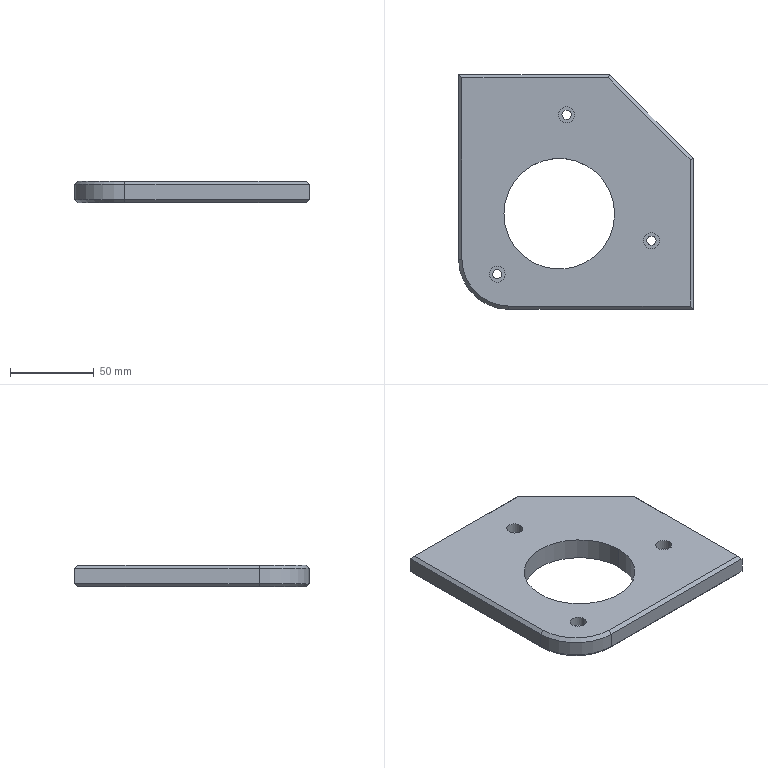Part | Creo | 1 solid | 37 faces | box 140 x 140 x 13 mm | volume 187737 mm3 | plane 20 | cylinder 15 | cone 2 | commonest cylinder face diameters 5.5 x6 9.5 x6 66 x2 60 x1
STEP:
#1=CARTESIAN_POINT('',(284.172,372.995,-24.));
#2=VERTEX_POINT('',#1);
#3=CARTESIAN_POINT('',(197.,372.995,-24.));
#4=VERTEX_POINT('',#3);
#5=CARTESIAN_POINT('',(284.172,372.995,-24.));
#6=DIRECTION('',(-1.,0.,0.));
#7=VECTOR('',#6,87.172);
#8=LINE('',#5,#7);
#9=EDGE_CURVE('',#2,#4,#8,.T.);
#10=ORIENTED_EDGE('',*,*,#9,.T.);
#11=CARTESIAN_POINT('',(197.,264.995,-24.));
#12=VERTEX_POINT('',#11);
#13=CARTESIAN_POINT('',(197.,372.995,-24.));
#14=DIRECTION('',(0.,-1.,0.));
#15=VECTOR('',#14,108.);
#16=LINE('',#13,#15);
#17=EDGE_CURVE('',#4,#12,#16,.T.);
#18=ORIENTED_EDGE('',*,*,#17,.T.);
#19=CARTESIAN_POINT('',(225.,236.995,-24.));
#20=VERTEX_POINT('',#19);
#21=CARTESIAN_POINT('',(225.,264.995,-24.));
#22=DIRECTION('',(0.,0.,-1.));
#23=DIRECTION('',(0.,-1.,0.));
#24=AXIS2_PLACEMENT_3D('',#21,#22,#23);
#25=CIRCLE('',#24,28.);
#26=EDGE_CURVE('',#20,#12,#25,.T.);
#27=ORIENTED_EDGE('',*,*,#26,.F.);
#28=CARTESIAN_POINT('',(333.,236.995,-24.));
#29=VERTEX_POINT('',#28);
#30=CARTESIAN_POINT('',(225.,236.995,-24.));
#31=DIRECTION('',(1.,0.,0.));
#32=VECTOR('',#31,108.);
#33=LINE('',#30,#32);
#34=EDGE_CURVE('',#20,#29,#33,.T.);
#35=ORIENTED_EDGE('',*,*,#34,.T.);
#36=CARTESIAN_POINT('',(333.,324.167,-24.));
#37=VERTEX_POINT('',#36);
#38=CARTESIAN_POINT('',(333.,236.995,-24.));
#39=DIRECTION('',(0.,1.,0.));
#40=VECTOR('',#39,87.172);
#41=LINE('',#38,#40);
#42=EDGE_CURVE('',#29,#37,#41,.T.);
#43=ORIENTED_EDGE('',*,*,#42,.T.);
#44=CARTESIAN_POINT('',(284.172,372.995,-24.));
#45=DIRECTION('',(0.7071,-0.7071,0.));
#46=VECTOR('',#45,69.054);
#47=LINE('',#44,#46);
#48=EDGE_CURVE('',#2,#37,#47,.T.);
#49=ORIENTED_EDGE('',*,*,#48,.F.);
#50=EDGE_LOOP('',(#10,#18,#27,#35,#43,#49));
#51=FACE_OUTER_BOUND('',#50,.F.);
#52=CARTESIAN_POINT('',(307.25,276.,-24.));
#53=VERTEX_POINT('',#52);
#54=CARTESIAN_POINT('',(312.75,276.,-24.));
#55=VERTEX_POINT('',#54);
#56=CARTESIAN_POINT('',(310.,276.,-24.));
#57=DIRECTION('',(0.,0.,1.));
#58=DIRECTION('',(-1.,0.,0.));
#59=AXIS2_PLACEMENT_3D('',#56,#57,#58);
#60=CIRCLE('',#59,2.75);
#61=EDGE_CURVE('',#53,#55,#60,.T.);
#62=ORIENTED_EDGE('',*,*,#61,.F.);
#63=CARTESIAN_POINT('',(310.,276.,-24.));
#64=DIRECTION('',(0.,0.,1.));
#65=DIRECTION('',(1.,0.,0.));
#66=AXIS2_PLACEMENT_3D('',#63,#64,#65);
#67=CIRCLE('',#66,2.75);
#68=EDGE_CURVE('',#55,#53,#67,.T.);
#69=ORIENTED_EDGE('',*,*,#68,.F.);
#70=EDGE_LOOP('',(#62,#69));
#71=FACE_BOUND('',#70,.F.);
#72=CARTESIAN_POINT('',(256.618,351.,-24.));
#73=VERTEX_POINT('',#72);
#74=CARTESIAN_POINT('',(262.118,351.,-24.));
#75=VERTEX_POINT('',#74);
#76=CARTESIAN_POINT('',(259.368,351.,-24.));
#77=DIRECTION('',(0.,0.,1.));
#78=DIRECTION('',(-1.,0.,0.));
#79=AXIS2_PLACEMENT_3D('',#76,#77,#78);
#80=CIRCLE('',#79,2.75);
#81=EDGE_CURVE('',#73,#75,#80,.T.);
#82=ORIENTED_EDGE('',*,*,#81,.F.);
#83=CARTESIAN_POINT('',(259.368,351.,-24.));
#84=DIRECTION('',(0.,0.,1.));
#85=DIRECTION('',(1.,0.,0.));
#86=AXIS2_PLACEMENT_3D('',#83,#84,#85);
#87=CIRCLE('',#86,2.75);
#88=EDGE_CURVE('',#75,#73,#87,.T.);
#89=ORIENTED_EDGE('',*,*,#88,.F.);
#90=EDGE_LOOP('',(#82,#89));
#91=FACE_BOUND('',#90,.F.);
#92=CARTESIAN_POINT('',(215.25,256.,-24.));
#93=VERTEX_POINT('',#92);
#94=CARTESIAN_POINT('',(220.75,256.,-24.));
#95=VERTEX_POINT('',#94);
#96=CARTESIAN_POINT('',(218.,256.,-24.));
#97=DIRECTION('',(0.,0.,1.));
#98=DIRECTION('',(-1.,0.,0.));
#99=AXIS2_PLACEMENT_3D('',#96,#97,#98);
#100=CIRCLE('',#99,2.75);
#101=EDGE_CURVE('',#93,#95,#100,.T.);
#102=ORIENTED_EDGE('',*,*,#101,.F.);
#103=CARTESIAN_POINT('',(218.,256.,-24.));
#104=DIRECTION('',(0.,0.,1.));
#105=DIRECTION('',(1.,0.,0.));
#106=AXIS2_PLACEMENT_3D('',#103,#104,#105);
#107=CIRCLE('',#106,2.75);
#108=EDGE_CURVE('',#95,#93,#107,.T.);
#109=ORIENTED_EDGE('',*,*,#108,.F.);
#110=EDGE_LOOP('',(#102,#109));
#111=FACE_BOUND('',#110,.F.);
#112=CARTESIAN_POINT('',(222.,291.995,-24.));
#113=VERTEX_POINT('',#112);
#114=CARTESIAN_POINT('',(288.,291.995,-24.));
#115=VERTEX_POINT('',#114);
#116=CARTESIAN_POINT('',(255.,291.995,-24.));
#117=DIRECTION('',(0.,0.,1.));
#118=DIRECTION('',(-1.,0.,0.));
#119=AXIS2_PLACEMENT_3D('',#116,#117,#118);
#120=CIRCLE('',#119,33.);
#121=EDGE_CURVE('',#113,#115,#120,.T.);
#122=ORIENTED_EDGE('',*,*,#121,.F.);
#123=CARTESIAN_POINT('',(255.,291.995,-24.));
#124=DIRECTION('',(0.,0.,1.));
#125=DIRECTION('',(1.,0.,0.));
#126=AXIS2_PLACEMENT_3D('',#123,#124,#125);
#127=CIRCLE('',#126,33.);
#128=EDGE_CURVE('',#115,#113,#127,.T.);
#129=ORIENTED_EDGE('',*,*,#128,.F.);
#130=EDGE_LOOP('',(#122,#129));
#131=FACE_BOUND('',#130,.F.);
#132=CARTESIAN_POINT('',(265.,302.495,-24.));
#133=DIRECTION('',(0.,0.,-1.));
#134=DIRECTION('',(-1.,0.,0.));
#135=AXIS2_PLACEMENT_3D('',#132,#133,#134);
#136=PLANE('',#135);
#137=ADVANCED_FACE('',(#51,#71,#91,#111,#131),#136,.T.);
#138=CARTESIAN_POINT('',(195.,374.995,-22.));
#139=VERTEX_POINT('',#138);
#140=CARTESIAN_POINT('',(195.,374.995,-22.));
#141=DIRECTION('',(0.5774,-0.5774,-0.5774));
#142=VECTOR('',#141,3.464);
#143=LINE('',#140,#142);
#144=EDGE_CURVE('',#139,#4,#143,.T.);
#145=ORIENTED_EDGE('',*,*,#144,.T.);
#146=ORIENTED_EDGE('',*,*,#9,.F.);
#147=CARTESIAN_POINT('',(285.,374.995,-22.));
#148=VERTEX_POINT('',#147);
#149=CARTESIAN_POINT('',(285.,374.995,-22.));
#150=DIRECTION('',(-0.2811,-0.6786,-0.6786));
#151=VECTOR('',#150,2.947);
#152=LINE('',#149,#151);
#153=EDGE_CURVE('',#148,#2,#152,.T.);
#154=ORIENTED_EDGE('',*,*,#153,.F.);
#155=CARTESIAN_POINT('',(195.,374.995,-22.));
#156=DIRECTION('',(1.,0.,0.));
#157=VECTOR('',#156,90.);
#158=LINE('',#155,#157);
#159=EDGE_CURVE('',#139,#148,#158,.T.);
#160=ORIENTED_EDGE('',*,*,#159,.F.);
#161=EDGE_LOOP('',(#145,#146,#154,#160));
#162=FACE_OUTER_BOUND('',#161,.F.);
#163=CARTESIAN_POINT('',(265.,372.995,-24.));
#164=DIRECTION('',(0.,-0.7071,0.7071));
#165=DIRECTION('',(1.,0.,0.));
#166=AXIS2_PLACEMENT_3D('',#163,#164,#165);
#167=PLANE('',#166);
#168=ADVANCED_FACE('',(#162),#167,.F.);
#169=CARTESIAN_POINT('',(195.,264.995,-22.));
#170=VERTEX_POINT('',#169);
#171=CARTESIAN_POINT('',(195.,264.995,-22.));
#172=DIRECTION('',(0.7071,0.,-0.7071));
#173=VECTOR('',#172,2.828);
#174=LINE('',#171,#173);
#175=EDGE_CURVE('',#170,#12,#174,.T.);
#176=ORIENTED_EDGE('',*,*,#175,.T.);
#177=ORIENTED_EDGE('',*,*,#17,.F.);
#178=ORIENTED_EDGE('',*,*,#144,.F.);
#179=CARTESIAN_POINT('',(195.,264.995,-22.));
#180=DIRECTION('',(0.,1.,0.));
#181=VECTOR('',#180,110.);
#182=LINE('',#179,#181);
#183=EDGE_CURVE('',#170,#139,#182,.T.);
#184=ORIENTED_EDGE('',*,*,#183,.F.);
#185=EDGE_LOOP('',(#176,#177,#178,#184));
#186=FACE_OUTER_BOUND('',#185,.F.);
#187=CARTESIAN_POINT('',(197.,302.495,-24.));
#188=DIRECTION('',(0.7071,0.,0.7071));
#189=DIRECTION('',(0.,1.,0.));
#190=AXIS2_PLACEMENT_3D('',#187,#188,#189);
#191=PLANE('',#190);
#192=ADVANCED_FACE('',(#186),#191,.F.);
#193=ORIENTED_EDGE('',*,*,#175,.F.);
#194=CARTESIAN_POINT('',(225.,234.995,-22.));
#195=VERTEX_POINT('',#194);
#196=CARTESIAN_POINT('',(225.,264.995,-22.));
#197=DIRECTION('',(0.,0.,-1.));
#198=DIRECTION('',(0.,-1.,0.));
#199=AXIS2_PLACEMENT_3D('',#196,#197,#198);
#200=CIRCLE('',#199,30.);
#201=EDGE_CURVE('',#195,#170,#200,.T.);
#202=ORIENTED_EDGE('',*,*,#201,.F.);
#203=CARTESIAN_POINT('',(225.,236.995,-24.));
#204=DIRECTION('',(0.,-0.7071,0.7071));
#205=VECTOR('',#204,2.828);
#206=LINE('',#203,#205);
#207=EDGE_CURVE('',#20,#195,#206,.T.);
#208=ORIENTED_EDGE('',*,*,#207,.F.);
#209=ORIENTED_EDGE('',*,*,#26,.T.);
#210=EDGE_LOOP('',(#193,#202,#208,#209));
#211=FACE_OUTER_BOUND('',#210,.F.);
#212=CARTESIAN_POINT('',(225.,264.995,-23.));
#213=DIRECTION('',(0.,0.,1.));
#214=DIRECTION('',(1.,0.,0.));
#215=AXIS2_PLACEMENT_3D('',#212,#213,#214);
#216=CONICAL_SURFACE('',#215,29.,45.);
#217=ADVANCED_FACE('',(#211),#216,.T.);
#218=CARTESIAN_POINT('',(225.,234.995,-13.));
#219=VERTEX_POINT('',#218);
#220=CARTESIAN_POINT('',(225.,234.995,-22.));
#221=DIRECTION('',(0.,0.,1.));
#222=VECTOR('',#221,9.);
#223=LINE('',#220,#222);
#224=EDGE_CURVE('',#195,#219,#223,.T.);
#225=ORIENTED_EDGE('',*,*,#224,.F.);
#226=ORIENTED_EDGE('',*,*,#201,.T.);
#227=CARTESIAN_POINT('',(195.,264.995,-13.));
#228=VERTEX_POINT('',#227);
#229=CARTESIAN_POINT('',(195.,264.995,-13.));
#230=DIRECTION('',(0.,0.,-1.));
#231=VECTOR('',#230,9.);
#232=LINE('',#229,#231);
#233=EDGE_CURVE('',#228,#170,#232,.T.);
#234=ORIENTED_EDGE('',*,*,#233,.F.);
#235=CARTESIAN_POINT('',(225.,264.995,-13.));
#236=DIRECTION('',(0.,0.,1.));
#237=DIRECTION('',(-1.,0.,0.));
#238=AXIS2_PLACEMENT_3D('',#235,#236,#237);
#239=CIRCLE('',#238,30.);
#240=EDGE_CURVE('',#228,#219,#239,.T.);
#241=ORIENTED_EDGE('',*,*,#240,.T.);
#242=EDGE_LOOP('',(#225,#226,#234,#241));
#243=FACE_OUTER_BOUND('',#242,.F.);
#244=CARTESIAN_POINT('',(225.,264.995,-11.));
#245=DIRECTION('',(0.,0.,-1.));
#246=DIRECTION('',(-1.,0.,0.));
#247=AXIS2_PLACEMENT_3D('',#244,#245,#246);
#248=CYLINDRICAL_SURFACE('',#247,30.);
#249=ADVANCED_FACE('',(#243),#248,.T.);
#250=CARTESIAN_POINT('',(335.,234.995,-22.));
#251=VERTEX_POINT('',#250);
#252=CARTESIAN_POINT('',(335.,234.995,-13.));
#253=VERTEX_POINT('',#252);
#254=CARTESIAN_POINT('',(335.,234.995,-22.));
#255=DIRECTION('',(0.,0.,1.));
#256=VECTOR('',#255,9.);
#257=LINE('',#254,#256);
#258=EDGE_CURVE('',#251,#253,#257,.T.);
#259=ORIENTED_EDGE('',*,*,#258,.F.);
#260=CARTESIAN_POINT('',(335.,234.995,-22.));
#261=DIRECTION('',(-1.,0.,0.));
#262=VECTOR('',#261,110.);
#263=LINE('',#260,#262);
#264=EDGE_CURVE('',#251,#195,#263,.T.);
#265=ORIENTED_EDGE('',*,*,#264,.T.);
#266=ORIENTED_EDGE('',*,*,#224,.T.);
#267=CARTESIAN_POINT('',(225.,234.995,-13.));
#268=DIRECTION('',(1.,0.,0.));
#269=VECTOR('',#268,110.);
#270=LINE('',#267,#269);
#271=EDGE_CURVE('',#219,#253,#270,.T.);
#272=ORIENTED_EDGE('',*,*,#271,.T.);
#273=EDGE_LOOP('',(#259,#265,#266,#272));
#274=FACE_OUTER_BOUND('',#273,.F.);
#275=CARTESIAN_POINT('',(265.,234.995,-11.));
#276=DIRECTION('',(0.,-1.,0.));
#277=DIRECTION('',(0.,0.,-1.));
#278=AXIS2_PLACEMENT_3D('',#275,#276,#277);
#279=PLANE('',#278);
#280=ADVANCED_FACE('',(#274),#279,.T.);
#281=CARTESIAN_POINT('',(335.,324.995,-13.));
#282=VERTEX_POINT('',#281);
#283=CARTESIAN_POINT('',(335.,324.995,-22.));
#284=VERTEX_POINT('',#283);
#285=CARTESIAN_POINT('',(335.,324.995,-13.));
#286=DIRECTION('',(0.,0.,-1.));
#287=VECTOR('',#286,9.);
#288=LINE('',#285,#287);
#289=EDGE_CURVE('',#282,#284,#288,.T.);
#290=ORIENTED_EDGE('',*,*,#289,.T.);
#291=CARTESIAN_POINT('',(335.,324.995,-22.));
#292=DIRECTION('',(0.,-1.,0.));
#293=VECTOR('',#292,90.);
#294=LINE('',#291,#293);
#295=EDGE_CURVE('',#284,#251,#294,.T.);
#296=ORIENTED_EDGE('',*,*,#295,.T.);
#297=ORIENTED_EDGE('',*,*,#258,.T.);
#298=CARTESIAN_POINT('',(335.,234.995,-13.));
#299=DIRECTION('',(0.,1.,0.));
#300=VECTOR('',#299,90.);
#301=LINE('',#298,#300);
#302=EDGE_CURVE('',#253,#282,#301,.T.);
#303=ORIENTED_EDGE('',*,*,#302,.T.);
#304=EDGE_LOOP('',(#290,#296,#297,#303));
#305=FACE_OUTER_BOUND('',#304,.F.);
#306=CARTESIAN_POINT('',(335.,-0.004699,-22.));
#307=DIRECTION('',(-1.,0.,0.));
#308=DIRECTION('',(0.,1.,0.));
#309=AXIS2_PLACEMENT_3D('',#306,#307,#308);
#310=PLANE('',#309);
#311=ADVANCED_FACE('',(#305),#310,.F.);
#312=CARTESIAN_POINT('',(285.,374.995,-13.));
#313=VERTEX_POINT('',#312);
#314=CARTESIAN_POINT('',(285.,374.995,-22.));
#315=DIRECTION('',(0.,0.,1.));
#316=VECTOR('',#315,9.);
#317=LINE('',#314,#316);
#318=EDGE_CURVE('',#148,#313,#317,.T.);
#319=ORIENTED_EDGE('',*,*,#318,.F.);
#320=CARTESIAN_POINT('',(285.,374.995,-22.));
#321=DIRECTION('',(0.7071,-0.7071,0.));
#322=VECTOR('',#321,70.711);
#323=LINE('',#320,#322);
#324=EDGE_CURVE('',#148,#284,#323,.T.);
#325=ORIENTED_EDGE('',*,*,#324,.T.);
#326=ORIENTED_EDGE('',*,*,#289,.F.);
#327=CARTESIAN_POINT('',(335.,324.995,-13.));
#328=DIRECTION('',(-0.7071,0.7071,0.));
#329=VECTOR('',#328,70.711);
#330=LINE('',#327,#329);
#331=EDGE_CURVE('',#282,#313,#330,.T.);
#332=ORIENTED_EDGE('',*,*,#331,.T.);
#333=EDGE_LOOP('',(#319,#325,#326,#332));
#334=FACE_OUTER_BOUND('',#333,.F.);
#335=CARTESIAN_POINT('',(285.,374.995,-187.));
#336=DIRECTION('',(0.7071,0.7071,0.));
#337=DIRECTION('',(0.,0.,1.));
#338=AXIS2_PLACEMENT_3D('',#335,#336,#337);
#339=PLANE('',#338);
#340=ADVANCED_FACE('',(#334),#339,.T.);
#341=CARTESIAN_POINT('',(195.,374.995,-13.));
#342=VERTEX_POINT('',#341);
#343=CARTESIAN_POINT('',(195.,374.995,-22.));
#344=DIRECTION('',(0.,0.,1.));
#345=VECTOR('',#344,9.);
#346=LINE('',#343,#345);
#347=EDGE_CURVE('',#139,#342,#346,.T.);
#348=ORIENTED_EDGE('',*,*,#347,.F.);
#349=ORIENTED_EDGE('',*,*,#159,.T.);
#350=ORIENTED_EDGE('',*,*,#318,.T.);
#351=CARTESIAN_POINT('',(285.,374.995,-13.));
#352=DIRECTION('',(-1.,0.,0.));
#353=VECTOR('',#352,90.);
#354=LINE('',#351,#353);
#355=EDGE_CURVE('',#313,#342,#354,.T.);
#356=ORIENTED_EDGE('',*,*,#355,.T.);
#357=EDGE_LOOP('',(#348,#349,#350,#356));
#358=FACE_OUTER_BOUND('',#357,.F.);
#359=CARTESIAN_POINT('',(285.,374.995,-187.));
#360=DIRECTION('',(0.,1.,0.));
#361=DIRECTION('',(0.,0.,1.));
#362=AXIS2_PLACEMENT_3D('',#359,#360,#361);
#363=PLANE('',#362);
#364=ADVANCED_FACE('',(#358),#363,.T.);
#365=ORIENTED_EDGE('',*,*,#233,.T.);
#366=ORIENTED_EDGE('',*,*,#183,.T.);
#367=ORIENTED_EDGE('',*,*,#347,.T.);
#368=CARTESIAN_POINT('',(195.,374.995,-13.));
#369=DIRECTION('',(0.,-1.,0.));
#370=VECTOR('',#369,110.);
#371=LINE('',#368,#370);
#372=EDGE_CURVE('',#342,#228,#371,.T.);
#373=ORIENTED_EDGE('',*,*,#372,.T.);
#374=EDGE_LOOP('',(#365,#366,#367,#373));
#375=FACE_OUTER_BOUND('',#374,.F.);
#376=CARTESIAN_POINT('',(195.,302.495,-11.));
#377=DIRECTION('',(-1.,0.,0.));
#378=DIRECTION('',(0.,0.,1.));
#379=AXIS2_PLACEMENT_3D('',#376,#377,#378);
#380=PLANE('',#379);
#381=ADVANCED_FACE('',(#375),#380,.T.);
#382=CARTESIAN_POINT('',(197.,264.995,-11.));
#383=VERTEX_POINT('',#382);
#384=CARTESIAN_POINT('',(197.,264.995,-11.));
#385=DIRECTION('',(-0.7071,0.,-0.7071));
#386=VECTOR('',#385,2.828);
#387=LINE('',#384,#386);
#388=EDGE_CURVE('',#383,#228,#387,.T.);
#389=ORIENTED_EDGE('',*,*,#388,.T.);
#390=ORIENTED_EDGE('',*,*,#372,.F.);
#391=CARTESIAN_POINT('',(197.,372.995,-11.));
#392=VERTEX_POINT('',#391);
#393=CARTESIAN_POINT('',(197.,372.995,-11.));
#394=DIRECTION('',(-0.5774,0.5774,-0.5774));
#395=VECTOR('',#394,3.464);
#396=LINE('',#393,#395);
#397=EDGE_CURVE('',#392,#342,#396,.T.);
#398=ORIENTED_EDGE('',*,*,#397,.F.);
#399=CARTESIAN_POINT('',(197.,264.995,-11.));
#400=DIRECTION('',(0.,1.,0.));
#401=VECTOR('',#400,108.);
#402=LINE('',#399,#401);
#403=EDGE_CURVE('',#383,#392,#402,.T.);
#404=ORIENTED_EDGE('',*,*,#403,.F.);
#405=EDGE_LOOP('',(#389,#390,#398,#404));
#406=FACE_OUTER_BOUND('',#405,.F.);
#407=CARTESIAN_POINT('',(197.,302.495,-11.));
#408=DIRECTION('',(0.7071,0.,-0.7071));
#409=DIRECTION('',(0.,-1.,0.));
#410=AXIS2_PLACEMENT_3D('',#407,#408,#409);
#411=PLANE('',#410);
#412=ADVANCED_FACE('',(#406),#411,.F.);
#413=ORIENTED_EDGE('',*,*,#388,.F.);
#414=CARTESIAN_POINT('',(225.,236.995,-11.));
#415=VERTEX_POINT('',#414);
#416=CARTESIAN_POINT('',(225.,264.995,-11.));
#417=DIRECTION('',(0.,0.,1.));
#418=DIRECTION('',(-1.,0.,0.));
#419=AXIS2_PLACEMENT_3D('',#416,#417,#418);
#420=CIRCLE('',#419,28.);
#421=EDGE_CURVE('',#383,#415,#420,.T.);
#422=ORIENTED_EDGE('',*,*,#421,.T.);
#423=CARTESIAN_POINT('',(225.,234.995,-13.));
#424=DIRECTION('',(0.,0.7071,0.7071));
#425=VECTOR('',#424,2.828);
#426=LINE('',#423,#425);
#427=EDGE_CURVE('',#219,#415,#426,.T.);
#428=ORIENTED_EDGE('',*,*,#427,.F.);
#429=ORIENTED_EDGE('',*,*,#240,.F.);
#430=EDGE_LOOP('',(#413,#422,#428,#429));
#431=FACE_OUTER_BOUND('',#430,.F.);
#432=CARTESIAN_POINT('',(225.,264.995,-12.));
#433=DIRECTION('',(0.,0.,-1.));
#434=DIRECTION('',(-1.,0.,0.));
#435=AXIS2_PLACEMENT_3D('',#432,#433,#434);
#436=CONICAL_SURFACE('',#435,29.,45.);
#437=ADVANCED_FACE('',(#431),#436,.T.);
#438=CARTESIAN_POINT('',(333.,324.167,-11.));
#439=VERTEX_POINT('',#438);
#440=CARTESIAN_POINT('',(333.,236.995,-11.));
#441=VERTEX_POINT('',#440);
#442=CARTESIAN_POINT('',(333.,324.167,-11.));
#443=DIRECTION('',(0.,-1.,0.));
#444=VECTOR('',#443,87.172);
#445=LINE('',#442,#444);
#446=EDGE_CURVE('',#439,#441,#445,.T.);
#447=ORIENTED_EDGE('',*,*,#446,.T.);
#448=CARTESIAN_POINT('',(333.,236.995,-11.));
#449=DIRECTION('',(-1.,0.,0.));
#450=VECTOR('',#449,108.);
#451=LINE('',#448,#450);
#452=EDGE_CURVE('',#441,#415,#451,.T.);
#453=ORIENTED_EDGE('',*,*,#452,.T.);
#454=ORIENTED_EDGE('',*,*,#421,.F.);
#455=ORIENTED_EDGE('',*,*,#403,.T.);
#456=CARTESIAN_POINT('',(284.172,372.995,-11.));
#457=VERTEX_POINT('',#456);
#458=CARTESIAN_POINT('',(197.,372.995,-11.));
#459=DIRECTION('',(1.,0.,0.));
#460=VECTOR('',#459,87.172);
#461=LINE('',#458,#460);
#462=EDGE_CURVE('',#392,#457,#461,.T.);
#463=ORIENTED_EDGE('',*,*,#462,.T.);
#464=CARTESIAN_POINT('',(333.,324.167,-11.));
#465=DIRECTION('',(-0.7071,0.7071,0.));
#466=VECTOR('',#465,69.054);
#467=LINE('',#464,#466);
#468=EDGE_CURVE('',#439,#457,#467,.T.);
#469=ORIENTED_EDGE('',*,*,#468,.F.);
#470=EDGE_LOOP('',(#447,#453,#454,#455,#463,#469));
#471=FACE_OUTER_BOUND('',#470,.F.);
#472=CARTESIAN_POINT('',(314.75,276.,-11.));
#473=VERTEX_POINT('',#472);
#474=CARTESIAN_POINT('',(305.25,276.,-11.));
#475=VERTEX_POINT('',#474);
#476=CARTESIAN_POINT('',(310.,276.,-11.));
#477=DIRECTION('',(0.,0.,-1.));
#478=DIRECTION('',(1.,0.,0.));
#479=AXIS2_PLACEMENT_3D('',#476,#477,#478);
#480=CIRCLE('',#479,4.75);
#481=EDGE_CURVE('',#473,#475,#480,.T.);
#482=ORIENTED_EDGE('',*,*,#481,.F.);
#483=CARTESIAN_POINT('',(310.,276.,-11.));
#484=DIRECTION('',(0.,0.,-1.));
#485=DIRECTION('',(-1.,0.,0.));
#486=AXIS2_PLACEMENT_3D('',#483,#484,#485);
#487=CIRCLE('',#486,4.75);
#488=EDGE_CURVE('',#475,#473,#487,.T.);
#489=ORIENTED_EDGE('',*,*,#488,.F.);
#490=EDGE_LOOP('',(#482,#489));
#491=FACE_BOUND('',#490,.F.);
#492=CARTESIAN_POINT('',(264.118,351.,-11.));
#493=VERTEX_POINT('',#492);
#494=CARTESIAN_POINT('',(254.618,351.,-11.));
#495=VERTEX_POINT('',#494);
#496=CARTESIAN_POINT('',(259.368,351.,-11.));
#497=DIRECTION('',(0.,0.,-1.));
#498=DIRECTION('',(1.,0.,0.));
#499=AXIS2_PLACEMENT_3D('',#496,#497,#498);
#500=CIRCLE('',#499,4.75);
#501=EDGE_CURVE('',#493,#495,#500,.T.);
#502=ORIENTED_EDGE('',*,*,#501,.F.);
#503=CARTESIAN_POINT('',(259.368,351.,-11.));
#504=DIRECTION('',(0.,0.,-1.));
#505=DIRECTION('',(-1.,0.,0.));
#506=AXIS2_PLACEMENT_3D('',#503,#504,#505);
#507=CIRCLE('',#506,4.75);
#508=EDGE_CURVE('',#495,#493,#507,.T.);
#509=ORIENTED_EDGE('',*,*,#508,.F.);
#510=EDGE_LOOP('',(#502,#509));
#511=FACE_BOUND('',#510,.F.);
#512=CARTESIAN_POINT('',(222.75,256.,-11.));
#513=VERTEX_POINT('',#512);
#514=CARTESIAN_POINT('',(213.25,256.,-11.));
#515=VERTEX_POINT('',#514);
#516=CARTESIAN_POINT('',(218.,256.,-11.));
#517=DIRECTION('',(0.,0.,-1.));
#518=DIRECTION('',(1.,0.,0.));
#519=AXIS2_PLACEMENT_3D('',#516,#517,#518);
#520=CIRCLE('',#519,4.75);
#521=EDGE_CURVE('',#513,#515,#520,.T.);
#522=ORIENTED_EDGE('',*,*,#521,.F.);
#523=CARTESIAN_POINT('',(218.,256.,-11.));
#524=DIRECTION('',(0.,0.,-1.));
#525=DIRECTION('',(-1.,0.,0.));
#526=AXIS2_PLACEMENT_3D('',#523,#524,#525);
#527=CIRCLE('',#526,4.75);
#528=EDGE_CURVE('',#515,#513,#527,.T.);
#529=ORIENTED_EDGE('',*,*,#528,.F.);
#530=EDGE_LOOP('',(#522,#529));
#531=FACE_BOUND('',#530,.F.);
#532=CARTESIAN_POINT('',(288.,291.995,-11.));
#533=VERTEX_POINT('',#532);
#534=CARTESIAN_POINT('',(222.,291.995,-11.));
#535=VERTEX_POINT('',#534);
#536=CARTESIAN_POINT('',(255.,291.995,-11.));
#537=DIRECTION('',(0.,0.,-1.));
#538=DIRECTION('',(1.,0.,0.));
#539=AXIS2_PLACEMENT_3D('',#536,#537,#538);
#540=CIRCLE('',#539,33.);
#541=EDGE_CURVE('',#533,#535,#540,.T.);
#542=ORIENTED_EDGE('',*,*,#541,.F.);
#543=CARTESIAN_POINT('',(255.,291.995,-11.));
#544=DIRECTION('',(0.,0.,-1.));
#545=DIRECTION('',(-1.,0.,0.));
#546=AXIS2_PLACEMENT_3D('',#543,#544,#545);
#547=CIRCLE('',#546,33.);
#548=EDGE_CURVE('',#535,#533,#547,.T.);
#549=ORIENTED_EDGE('',*,*,#548,.F.);
#550=EDGE_LOOP('',(#542,#549));
#551=FACE_BOUND('',#550,.F.);
#552=CARTESIAN_POINT('',(265.,302.495,-11.));
#553=DIRECTION('',(0.,0.,1.));
#554=DIRECTION('',(1.,0.,0.));
#555=AXIS2_PLACEMENT_3D('',#552,#553,#554);
#556=PLANE('',#555);
#557=ADVANCED_FACE('',(#471,#491,#511,#531,#551),#556,.T.);
#558=CARTESIAN_POINT('',(335.,234.995,-13.));
#559=DIRECTION('',(-0.5774,0.5774,0.5774));
#560=VECTOR('',#559,3.464);
#561=LINE('',#558,#560);
#562=EDGE_CURVE('',#253,#441,#561,.T.);
#563=ORIENTED_EDGE('',*,*,#562,.T.);
#564=ORIENTED_EDGE('',*,*,#446,.F.);
#565=CARTESIAN_POINT('',(335.,324.995,-13.));
#566=DIRECTION('',(-0.6786,-0.2811,0.6786));
#567=VECTOR('',#566,2.947);
#568=LINE('',#565,#567);
#569=EDGE_CURVE('',#282,#439,#568,.T.);
#570=ORIENTED_EDGE('',*,*,#569,.F.);
#571=ORIENTED_EDGE('',*,*,#302,.F.);
#572=EDGE_LOOP('',(#563,#564,#570,#571));
#573=FACE_OUTER_BOUND('',#572,.F.);
#574=CARTESIAN_POINT('',(333.,302.495,-11.));
#575=DIRECTION('',(0.7071,0.,0.7071));
#576=DIRECTION('',(0.,-1.,0.));
#577=AXIS2_PLACEMENT_3D('',#574,#575,#576);
#578=PLANE('',#577);
#579=ADVANCED_FACE('',(#573),#578,.T.);
#580=ORIENTED_EDGE('',*,*,#427,.T.);
#581=ORIENTED_EDGE('',*,*,#452,.F.);
#582=ORIENTED_EDGE('',*,*,#562,.F.);
#583=ORIENTED_EDGE('',*,*,#271,.F.);
#584=EDGE_LOOP('',(#580,#581,#582,#583));
#585=FACE_OUTER_BOUND('',#584,.F.);
#586=CARTESIAN_POINT('',(265.,236.995,-11.));
#587=DIRECTION('',(0.,0.7071,-0.7071));
#588=DIRECTION('',(1.,0.,0.));
#589=AXIS2_PLACEMENT_3D('',#586,#587,#588);
#590=PLANE('',#589);
#591=ADVANCED_FACE('',(#585),#590,.F.);
#592=ORIENTED_EDGE('',*,*,#569,.T.);
#593=ORIENTED_EDGE('',*,*,#468,.T.);
#594=CARTESIAN_POINT('',(284.172,372.995,-11.));
#595=DIRECTION('',(0.2811,0.6786,-0.6786));
#596=VECTOR('',#595,2.947);
#597=LINE('',#594,#596);
#598=EDGE_CURVE('',#457,#313,#597,.T.);
#599=ORIENTED_EDGE('',*,*,#598,.T.);
#600=ORIENTED_EDGE('',*,*,#331,.F.);
#601=EDGE_LOOP('',(#592,#593,#599,#600));
#602=FACE_OUTER_BOUND('',#601,.F.);
#603=CARTESIAN_POINT('',(309.836,347.331,-11.));
#604=DIRECTION('',(-0.5,-0.5,-0.7071));
#605=DIRECTION('',(-0.7071,0.7071,0.));
#606=AXIS2_PLACEMENT_3D('',#603,#604,#605);
#607=PLANE('',#606);
#608=ADVANCED_FACE('',(#602),#607,.F.);
#609=ORIENTED_EDGE('',*,*,#397,.T.);
#610=ORIENTED_EDGE('',*,*,#355,.F.);
#611=ORIENTED_EDGE('',*,*,#598,.F.);
#612=ORIENTED_EDGE('',*,*,#462,.F.);
#613=EDGE_LOOP('',(#609,#610,#611,#612));
#614=FACE_OUTER_BOUND('',#613,.F.);
#615=CARTESIAN_POINT('',(265.,372.995,-11.));
#616=DIRECTION('',(0.,-0.7071,-0.7071));
#617=DIRECTION('',(-1.,0.,0.));
#618=AXIS2_PLACEMENT_3D('',#615,#616,#617);
#619=PLANE('',#618);
#620=ADVANCED_FACE('',(#614),#619,.F.);
#621=CARTESIAN_POINT('',(305.25,276.,-17.));
#622=VERTEX_POINT('',#621);
#623=CARTESIAN_POINT('',(314.75,276.,-17.));
#624=VERTEX_POINT('',#623);
#625=CARTESIAN_POINT('',(310.,276.,-17.));
#626=DIRECTION('',(0.,0.,1.));
#627=DIRECTION('',(-1.,0.,0.));
#628=AXIS2_PLACEMENT_3D('',#625,#626,#627);
#629=CIRCLE('',#628,4.75);
#630=EDGE_CURVE('',#622,#624,#629,.T.);
#631=ORIENTED_EDGE('',*,*,#630,.T.);
#632=CARTESIAN_POINT('',(314.75,276.,-17.));
#633=DIRECTION('',(0.,0.,1.));
#634=VECTOR('',#633,6.);
#635=LINE('',#632,#634);
#636=EDGE_CURVE('',#624,#473,#635,.T.);
#637=ORIENTED_EDGE('',*,*,#636,.T.);
#638=ORIENTED_EDGE('',*,*,#481,.T.);
#639=CARTESIAN_POINT('',(305.25,276.,-17.));
#640=DIRECTION('',(0.,0.,1.));
#641=VECTOR('',#640,6.);
#642=LINE('',#639,#641);
#643=EDGE_CURVE('',#622,#475,#642,.T.);
#644=ORIENTED_EDGE('',*,*,#643,.F.);
#645=EDGE_LOOP('',(#631,#637,#638,#644));
#646=FACE_OUTER_BOUND('',#645,.F.);
#647=CARTESIAN_POINT('',(310.,276.,-11.));
#648=DIRECTION('',(0.,0.,1.));
#649=DIRECTION('',(1.,0.,0.));
#650=AXIS2_PLACEMENT_3D('',#647,#648,#649);
#651=CYLINDRICAL_SURFACE('',#650,4.75);
#652=ADVANCED_FACE('',(#646),#651,.F.);
#653=CARTESIAN_POINT('',(310.,276.,-17.));
#654=DIRECTION('',(0.,0.,1.));
#655=DIRECTION('',(1.,0.,0.));
#656=AXIS2_PLACEMENT_3D('',#653,#654,#655);
#657=CIRCLE('',#656,4.75);
#658=EDGE_CURVE('',#624,#622,#657,.T.);
#659=ORIENTED_EDGE('',*,*,#658,.F.);
#660=ORIENTED_EDGE('',*,*,#630,.F.);
#661=EDGE_LOOP('',(#659,#660));
#662=FACE_OUTER_BOUND('',#661,.F.);
#663=CARTESIAN_POINT('',(312.75,276.,-17.));
#664=VERTEX_POINT('',#663);
#665=CARTESIAN_POINT('',(307.25,276.,-17.));
#666=VERTEX_POINT('',#665);
#667=CARTESIAN_POINT('',(310.,276.,-17.));
#668=DIRECTION('',(0.,0.,-1.));
#669=DIRECTION('',(1.,0.,0.));
#670=AXIS2_PLACEMENT_3D('',#667,#668,#669);
#671=CIRCLE('',#670,2.75);
#672=EDGE_CURVE('',#664,#666,#671,.T.);
#673=ORIENTED_EDGE('',*,*,#672,.F.);
#674=CARTESIAN_POINT('',(310.,276.,-17.));
#675=DIRECTION('',(0.,0.,-1.));
#676=DIRECTION('',(-1.,0.,0.));
#677=AXIS2_PLACEMENT_3D('',#674,#675,#676);
#678=CIRCLE('',#677,2.75);
#679=EDGE_CURVE('',#666,#664,#678,.T.);
#680=ORIENTED_EDGE('',*,*,#679,.F.);
#681=EDGE_LOOP('',(#673,#680));
#682=FACE_BOUND('',#681,.F.);
#683=CARTESIAN_POINT('',(310.,280.75,-17.));
#684=DIRECTION('',(0.,0.,-1.));
#685=DIRECTION('',(-1.,0.,0.));
#686=AXIS2_PLACEMENT_3D('',#683,#684,#685);
#687=PLANE('',#686);
#688=ADVANCED_FACE('',(#662,#682),#687,.F.);
#689=ORIENTED_EDGE('',*,*,#61,.T.);
#690=CARTESIAN_POINT('',(312.75,276.,-24.));
#691=DIRECTION('',(0.,0.,1.));
#692=VECTOR('',#691,7.);
#693=LINE('',#690,#692);
#694=EDGE_CURVE('',#55,#664,#693,.T.);
#695=ORIENTED_EDGE('',*,*,#694,.T.);
#696=ORIENTED_EDGE('',*,*,#672,.T.);
#697=CARTESIAN_POINT('',(307.25,276.,-24.));
#698=DIRECTION('',(0.,0.,1.));
#699=VECTOR('',#698,7.);
#700=LINE('',#697,#699);
#701=EDGE_CURVE('',#53,#666,#700,.T.);
#702=ORIENTED_EDGE('',*,*,#701,.F.);
#703=EDGE_LOOP('',(#689,#695,#696,#702));
#704=FACE_OUTER_BOUND('',#703,.F.);
#705=CARTESIAN_POINT('',(310.,276.,-11.));
#706=DIRECTION('',(0.,0.,1.));
#707=DIRECTION('',(1.,0.,0.));
#708=AXIS2_PLACEMENT_3D('',#705,#706,#707);
#709=CYLINDRICAL_SURFACE('',#708,2.75);
#710=ADVANCED_FACE('',(#704),#709,.F.);
#711=ORIENTED_EDGE('',*,*,#68,.T.);
#712=ORIENTED_EDGE('',*,*,#701,.T.);
#713=ORIENTED_EDGE('',*,*,#679,.T.);
#714=ORIENTED_EDGE('',*,*,#694,.F.);
#715=EDGE_LOOP('',(#711,#712,#713,#714));
#716=FACE_OUTER_BOUND('',#715,.F.);
#717=CARTESIAN_POINT('',(310.,276.,-11.));
#718=DIRECTION('',(0.,0.,1.));
#719=DIRECTION('',(1.,0.,0.));
#720=AXIS2_PLACEMENT_3D('',#717,#718,#719);
#721=CYLINDRICAL_SURFACE('',#720,2.75);
#722=ADVANCED_FACE('',(#716),#721,.F.);
#723=ORIENTED_EDGE('',*,*,#658,.T.);
#724=ORIENTED_EDGE('',*,*,#643,.T.);
#725=ORIENTED_EDGE('',*,*,#488,.T.);
#726=ORIENTED_EDGE('',*,*,#636,.F.);
#727=EDGE_LOOP('',(#723,#724,#725,#726));
#728=FACE_OUTER_BOUND('',#727,.F.);
#729=CARTESIAN_POINT('',(310.,276.,-11.));
#730=DIRECTION('',(0.,0.,1.));
#731=DIRECTION('',(1.,0.,0.));
#732=AXIS2_PLACEMENT_3D('',#729,#730,#731);
#733=CYLINDRICAL_SURFACE('',#732,4.75);
#734=ADVANCED_FACE('',(#728),#733,.F.);
#735=CARTESIAN_POINT('',(254.618,351.,-17.));
#736=VERTEX_POINT('',#735);
#737=CARTESIAN_POINT('',(264.118,351.,-17.));
#738=VERTEX_POINT('',#737);
#739=CARTESIAN_POINT('',(259.368,351.,-17.));
#740=DIRECTION('',(0.,0.,1.));
#741=DIRECTION('',(-1.,0.,0.));
#742=AXIS2_PLACEMENT_3D('',#739,#740,#741);
#743=CIRCLE('',#742,4.75);
#744=EDGE_CURVE('',#736,#738,#743,.T.);
#745=ORIENTED_EDGE('',*,*,#744,.T.);
#746=CARTESIAN_POINT('',(264.118,351.,-17.));
#747=DIRECTION('',(0.,0.,1.));
#748=VECTOR('',#747,6.);
#749=LINE('',#746,#748);
#750=EDGE_CURVE('',#738,#493,#749,.T.);
#751=ORIENTED_EDGE('',*,*,#750,.T.);
#752=ORIENTED_EDGE('',*,*,#501,.T.);
#753=CARTESIAN_POINT('',(254.618,351.,-17.));
#754=DIRECTION('',(0.,0.,1.));
#755=VECTOR('',#754,6.);
#756=LINE('',#753,#755);
#757=EDGE_CURVE('',#736,#495,#756,.T.);
#758=ORIENTED_EDGE('',*,*,#757,.F.);
#759=EDGE_LOOP('',(#745,#751,#752,#758));
#760=FACE_OUTER_BOUND('',#759,.F.);
#761=CARTESIAN_POINT('',(259.368,351.,-11.));
#762=DIRECTION('',(0.,0.,1.));
#763=DIRECTION('',(1.,0.,0.));
#764=AXIS2_PLACEMENT_3D('',#761,#762,#763);
#765=CYLINDRICAL_SURFACE('',#764,4.75);
#766=ADVANCED_FACE('',(#760),#765,.F.);
#767=CARTESIAN_POINT('',(259.368,351.,-17.));
#768=DIRECTION('',(0.,0.,1.));
#769=DIRECTION('',(1.,0.,0.));
#770=AXIS2_PLACEMENT_3D('',#767,#768,#769);
#771=CIRCLE('',#770,4.75);
#772=EDGE_CURVE('',#738,#736,#771,.T.);
#773=ORIENTED_EDGE('',*,*,#772,.F.);
#774=ORIENTED_EDGE('',*,*,#744,.F.);
#775=EDGE_LOOP('',(#773,#774));
#776=FACE_OUTER_BOUND('',#775,.F.);
#777=CARTESIAN_POINT('',(262.118,351.,-17.));
#778=VERTEX_POINT('',#777);
#779=CARTESIAN_POINT('',(256.618,351.,-17.));
#780=VERTEX_POINT('',#779);
#781=CARTESIAN_POINT('',(259.368,351.,-17.));
#782=DIRECTION('',(0.,0.,-1.));
#783=DIRECTION('',(1.,0.,0.));
#784=AXIS2_PLACEMENT_3D('',#781,#782,#783);
#785=CIRCLE('',#784,2.75);
#786=EDGE_CURVE('',#778,#780,#785,.T.);
#787=ORIENTED_EDGE('',*,*,#786,.F.);
#788=CARTESIAN_POINT('',(259.368,351.,-17.));
#789=DIRECTION('',(0.,0.,-1.));
#790=DIRECTION('',(-1.,0.,0.));
#791=AXIS2_PLACEMENT_3D('',#788,#789,#790);
#792=CIRCLE('',#791,2.75);
#793=EDGE_CURVE('',#780,#778,#792,.T.);
#794=ORIENTED_EDGE('',*,*,#793,.F.);
#795=EDGE_LOOP('',(#787,#794));
#796=FACE_BOUND('',#795,.F.);
#797=CARTESIAN_POINT('',(259.368,355.75,-17.));
#798=DIRECTION('',(0.,0.,-1.));
#799=DIRECTION('',(-1.,0.,0.));
#800=AXIS2_PLACEMENT_3D('',#797,#798,#799);
#801=PLANE('',#800);
#802=ADVANCED_FACE('',(#776,#796),#801,.F.);
#803=ORIENTED_EDGE('',*,*,#81,.T.);
#804=CARTESIAN_POINT('',(262.118,351.,-24.));
#805=DIRECTION('',(0.,0.,1.));
#806=VECTOR('',#805,7.);
#807=LINE('',#804,#806);
#808=EDGE_CURVE('',#75,#778,#807,.T.);
#809=ORIENTED_EDGE('',*,*,#808,.T.);
#810=ORIENTED_EDGE('',*,*,#786,.T.);
#811=CARTESIAN_POINT('',(256.618,351.,-24.));
#812=DIRECTION('',(0.,0.,1.));
#813=VECTOR('',#812,7.);
#814=LINE('',#811,#813);
#815=EDGE_CURVE('',#73,#780,#814,.T.);
#816=ORIENTED_EDGE('',*,*,#815,.F.);
#817=EDGE_LOOP('',(#803,#809,#810,#816));
#818=FACE_OUTER_BOUND('',#817,.F.);
#819=CARTESIAN_POINT('',(259.368,351.,-11.));
#820=DIRECTION('',(0.,0.,1.));
#821=DIRECTION('',(1.,0.,0.));
#822=AXIS2_PLACEMENT_3D('',#819,#820,#821);
#823=CYLINDRICAL_SURFACE('',#822,2.75);
#824=ADVANCED_FACE('',(#818),#823,.F.);
#825=ORIENTED_EDGE('',*,*,#88,.T.);
#826=ORIENTED_EDGE('',*,*,#815,.T.);
#827=ORIENTED_EDGE('',*,*,#793,.T.);
#828=ORIENTED_EDGE('',*,*,#808,.F.);
#829=EDGE_LOOP('',(#825,#826,#827,#828));
#830=FACE_OUTER_BOUND('',#829,.F.);
#831=CARTESIAN_POINT('',(259.368,351.,-11.));
#832=DIRECTION('',(0.,0.,1.));
#833=DIRECTION('',(1.,0.,0.));
#834=AXIS2_PLACEMENT_3D('',#831,#832,#833);
#835=CYLINDRICAL_SURFACE('',#834,2.75);
#836=ADVANCED_FACE('',(#830),#835,.F.);
#837=ORIENTED_EDGE('',*,*,#772,.T.);
#838=ORIENTED_EDGE('',*,*,#757,.T.);
#839=ORIENTED_EDGE('',*,*,#508,.T.);
#840=ORIENTED_EDGE('',*,*,#750,.F.);
#841=EDGE_LOOP('',(#837,#838,#839,#840));
#842=FACE_OUTER_BOUND('',#841,.F.);
#843=CARTESIAN_POINT('',(259.368,351.,-11.));
#844=DIRECTION('',(0.,0.,1.));
#845=DIRECTION('',(1.,0.,0.));
#846=AXIS2_PLACEMENT_3D('',#843,#844,#845);
#847=CYLINDRICAL_SURFACE('',#846,4.75);
#848=ADVANCED_FACE('',(#842),#847,.F.);
#849=CARTESIAN_POINT('',(213.25,256.,-17.));
#850=VERTEX_POINT('',#849);
#851=CARTESIAN_POINT('',(222.75,256.,-17.));
#852=VERTEX_POINT('',#851);
#853=CARTESIAN_POINT('',(218.,256.,-17.));
#854=DIRECTION('',(0.,0.,1.));
#855=DIRECTION('',(-1.,0.,0.));
#856=AXIS2_PLACEMENT_3D('',#853,#854,#855);
#857=CIRCLE('',#856,4.75);
#858=EDGE_CURVE('',#850,#852,#857,.T.);
#859=ORIENTED_EDGE('',*,*,#858,.T.);
#860=CARTESIAN_POINT('',(222.75,256.,-17.));
#861=DIRECTION('',(0.,0.,1.));
#862=VECTOR('',#861,6.);
#863=LINE('',#860,#862);
#864=EDGE_CURVE('',#852,#513,#863,.T.);
#865=ORIENTED_EDGE('',*,*,#864,.T.);
#866=ORIENTED_EDGE('',*,*,#521,.T.);
#867=CARTESIAN_POINT('',(213.25,256.,-17.));
#868=DIRECTION('',(0.,0.,1.));
#869=VECTOR('',#868,6.);
#870=LINE('',#867,#869);
#871=EDGE_CURVE('',#850,#515,#870,.T.);
#872=ORIENTED_EDGE('',*,*,#871,.F.);
#873=EDGE_LOOP('',(#859,#865,#866,#872));
#874=FACE_OUTER_BOUND('',#873,.F.);
#875=CARTESIAN_POINT('',(218.,256.,-11.));
#876=DIRECTION('',(0.,0.,1.));
#877=DIRECTION('',(1.,0.,0.));
#878=AXIS2_PLACEMENT_3D('',#875,#876,#877);
#879=CYLINDRICAL_SURFACE('',#878,4.75);
#880=ADVANCED_FACE('',(#874),#879,.F.);
#881=CARTESIAN_POINT('',(218.,256.,-17.));
#882=DIRECTION('',(0.,0.,1.));
#883=DIRECTION('',(1.,0.,0.));
#884=AXIS2_PLACEMENT_3D('',#881,#882,#883);
#885=CIRCLE('',#884,4.75);
#886=EDGE_CURVE('',#852,#850,#885,.T.);
#887=ORIENTED_EDGE('',*,*,#886,.F.);
#888=ORIENTED_EDGE('',*,*,#858,.F.);
#889=EDGE_LOOP('',(#887,#888));
#890=FACE_OUTER_BOUND('',#889,.F.);
#891=CARTESIAN_POINT('',(220.75,256.,-17.));
#892=VERTEX_POINT('',#891);
#893=CARTESIAN_POINT('',(215.25,256.,-17.));
#894=VERTEX_POINT('',#893);
#895=CARTESIAN_POINT('',(218.,256.,-17.));
#896=DIRECTION('',(0.,0.,-1.));
#897=DIRECTION('',(1.,0.,0.));
#898=AXIS2_PLACEMENT_3D('',#895,#896,#897);
#899=CIRCLE('',#898,2.75);
#900=EDGE_CURVE('',#892,#894,#899,.T.);
#901=ORIENTED_EDGE('',*,*,#900,.F.);
#902=CARTESIAN_POINT('',(218.,256.,-17.));
#903=DIRECTION('',(0.,0.,-1.));
#904=DIRECTION('',(-1.,0.,0.));
#905=AXIS2_PLACEMENT_3D('',#902,#903,#904);
#906=CIRCLE('',#905,2.75);
#907=EDGE_CURVE('',#894,#892,#906,.T.);
#908=ORIENTED_EDGE('',*,*,#907,.F.);
#909=EDGE_LOOP('',(#901,#908));
#910=FACE_BOUND('',#909,.F.);
#911=CARTESIAN_POINT('',(218.,260.75,-17.));
#912=DIRECTION('',(0.,0.,-1.));
#913=DIRECTION('',(-1.,0.,0.));
#914=AXIS2_PLACEMENT_3D('',#911,#912,#913);
#915=PLANE('',#914);
#916=ADVANCED_FACE('',(#890,#910),#915,.F.);
#917=ORIENTED_EDGE('',*,*,#101,.T.);
#918=CARTESIAN_POINT('',(220.75,256.,-24.));
#919=DIRECTION('',(0.,0.,1.));
#920=VECTOR('',#919,7.);
#921=LINE('',#918,#920);
#922=EDGE_CURVE('',#95,#892,#921,.T.);
#923=ORIENTED_EDGE('',*,*,#922,.T.);
#924=ORIENTED_EDGE('',*,*,#900,.T.);
#925=CARTESIAN_POINT('',(215.25,256.,-24.));
#926=DIRECTION('',(0.,0.,1.));
#927=VECTOR('',#926,7.);
#928=LINE('',#925,#927);
#929=EDGE_CURVE('',#93,#894,#928,.T.);
#930=ORIENTED_EDGE('',*,*,#929,.F.);
#931=EDGE_LOOP('',(#917,#923,#924,#930));
#932=FACE_OUTER_BOUND('',#931,.F.);
#933=CARTESIAN_POINT('',(218.,256.,-11.));
#934=DIRECTION('',(0.,0.,1.));
#935=DIRECTION('',(1.,0.,0.));
#936=AXIS2_PLACEMENT_3D('',#933,#934,#935);
#937=CYLINDRICAL_SURFACE('',#936,2.75);
#938=ADVANCED_FACE('',(#932),#937,.F.);
#939=ORIENTED_EDGE('',*,*,#108,.T.);
#940=ORIENTED_EDGE('',*,*,#929,.T.);
#941=ORIENTED_EDGE('',*,*,#907,.T.);
#942=ORIENTED_EDGE('',*,*,#922,.F.);
#943=EDGE_LOOP('',(#939,#940,#941,#942));
#944=FACE_OUTER_BOUND('',#943,.F.);
#945=CARTESIAN_POINT('',(218.,256.,-11.));
#946=DIRECTION('',(0.,0.,1.));
#947=DIRECTION('',(1.,0.,0.));
#948=AXIS2_PLACEMENT_3D('',#945,#946,#947);
#949=CYLINDRICAL_SURFACE('',#948,2.75);
#950=ADVANCED_FACE('',(#944),#949,.F.);
#951=ORIENTED_EDGE('',*,*,#886,.T.);
#952=ORIENTED_EDGE('',*,*,#871,.T.);
#953=ORIENTED_EDGE('',*,*,#528,.T.);
#954=ORIENTED_EDGE('',*,*,#864,.F.);
#955=EDGE_LOOP('',(#951,#952,#953,#954));
#956=FACE_OUTER_BOUND('',#955,.F.);
#957=CARTESIAN_POINT('',(218.,256.,-11.));
#958=DIRECTION('',(0.,0.,1.));
#959=DIRECTION('',(1.,0.,0.));
#960=AXIS2_PLACEMENT_3D('',#957,#958,#959);
#961=CYLINDRICAL_SURFACE('',#960,4.75);
#962=ADVANCED_FACE('',(#956),#961,.F.);
#963=ORIENTED_EDGE('',*,*,#541,.T.);
#964=CARTESIAN_POINT('',(222.,291.995,-11.));
#965=DIRECTION('',(0.,0.,-1.));
#966=VECTOR('',#965,13.);
#967=LINE('',#964,#966);
#968=EDGE_CURVE('',#535,#113,#967,.T.);
#969=ORIENTED_EDGE('',*,*,#968,.T.);
#970=ORIENTED_EDGE('',*,*,#121,.T.);
#971=CARTESIAN_POINT('',(288.,291.995,-11.));
#972=DIRECTION('',(0.,0.,-1.));
#973=VECTOR('',#972,13.);
#974=LINE('',#971,#973);
#975=EDGE_CURVE('',#533,#115,#974,.T.);
#976=ORIENTED_EDGE('',*,*,#975,.F.);
#977=EDGE_LOOP('',(#963,#969,#970,#976));
#978=FACE_OUTER_BOUND('',#977,.F.);
#979=CARTESIAN_POINT('',(255.,291.995,-201.));
#980=DIRECTION('',(0.,0.,-1.));
#981=DIRECTION('',(1.,0.,0.));
#982=AXIS2_PLACEMENT_3D('',#979,#980,#981);
#983=CYLINDRICAL_SURFACE('',#982,33.);
#984=ADVANCED_FACE('',(#978),#983,.F.);
#985=ORIENTED_EDGE('',*,*,#548,.T.);
#986=ORIENTED_EDGE('',*,*,#975,.T.);
#987=ORIENTED_EDGE('',*,*,#128,.T.);
#988=ORIENTED_EDGE('',*,*,#968,.F.);
#989=EDGE_LOOP('',(#985,#986,#987,#988));
#990=FACE_OUTER_BOUND('',#989,.F.);
#991=CARTESIAN_POINT('',(255.,291.995,-201.));
#992=DIRECTION('',(0.,0.,-1.));
#993=DIRECTION('',(1.,0.,0.));
#994=AXIS2_PLACEMENT_3D('',#991,#992,#993);
#995=CYLINDRICAL_SURFACE('',#994,33.);
#996=ADVANCED_FACE('',(#990),#995,.F.);
#997=ORIENTED_EDGE('',*,*,#153,.T.);
#998=ORIENTED_EDGE('',*,*,#48,.T.);
#999=CARTESIAN_POINT('',(335.,324.995,-22.));
#1000=DIRECTION('',(-0.6786,-0.2811,-0.6786));
#1001=VECTOR('',#1000,2.947);
#1002=LINE('',#999,#1001);
#1003=EDGE_CURVE('',#284,#37,#1002,.T.);
#1004=ORIENTED_EDGE('',*,*,#1003,.F.);
#1005=ORIENTED_EDGE('',*,*,#324,.F.);
#1006=EDGE_LOOP('',(#997,#998,#1004,#1005));
#1007=FACE_OUTER_BOUND('',#1006,.F.);
#1008=CARTESIAN_POINT('',(309.836,347.331,-24.));
#1009=DIRECTION('',(-0.5,-0.5,0.7071));
#1010=DIRECTION('',(0.7071,-0.7071,0.));
#1011=AXIS2_PLACEMENT_3D('',#1008,#1009,#1010);
#1012=PLANE('',#1011);
#1013=ADVANCED_FACE('',(#1007),#1012,.F.);
#1014=ORIENTED_EDGE('',*,*,#1003,.T.);
#1015=ORIENTED_EDGE('',*,*,#42,.F.);
#1016=CARTESIAN_POINT('',(333.,236.995,-24.));
#1017=DIRECTION('',(0.5774,-0.5774,0.5774));
#1018=VECTOR('',#1017,3.464);
#1019=LINE('',#1016,#1018);
#1020=EDGE_CURVE('',#29,#251,#1019,.T.);
#1021=ORIENTED_EDGE('',*,*,#1020,.T.);
#1022=ORIENTED_EDGE('',*,*,#295,.F.);
#1023=EDGE_LOOP('',(#1014,#1015,#1021,#1022));
#1024=FACE_OUTER_BOUND('',#1023,.F.);
#1025=CARTESIAN_POINT('',(333.,302.495,-24.));
#1026=DIRECTION('',(0.7071,0.,-0.7071));
#1027=DIRECTION('',(0.,1.,0.));
#1028=AXIS2_PLACEMENT_3D('',#1025,#1026,#1027);
#1029=PLANE('',#1028);
#1030=ADVANCED_FACE('',(#1024),#1029,.T.);
#1031=ORIENTED_EDGE('',*,*,#207,.T.);
#1032=ORIENTED_EDGE('',*,*,#264,.F.);
#1033=ORIENTED_EDGE('',*,*,#1020,.F.);
#1034=ORIENTED_EDGE('',*,*,#34,.F.);
#1035=EDGE_LOOP('',(#1031,#1032,#1033,#1034));
#1036=FACE_OUTER_BOUND('',#1035,.F.);
#1037=CARTESIAN_POINT('',(265.,236.995,-24.));
#1038=DIRECTION('',(0.,0.7071,0.7071));
#1039=DIRECTION('',(-1.,0.,0.));
#1040=AXIS2_PLACEMENT_3D('',#1037,#1038,#1039);
#1041=PLANE('',#1040);
#1042=ADVANCED_FACE('',(#1036),#1041,.F.);
#1043=CLOSED_SHELL('',(#137,#168,#192,#217,#249,#280,#311,#340,#364,#381,#412,#437,#557,#579,#591,#608,#620,#652,#688,#710,#722,#734,#766,#802,#824,#836,#848,#880,#916,#938,#950,#962,#984,#996,#1013,#1030,#1042));
#1044=MANIFOLD_SOLID_BREP('',#1043);
#1045=(LENGTH_UNIT()NAMED_UNIT(*)SI_UNIT(.MILLI.,.METRE.));
#1046=UNCERTAINTY_MEASURE_WITH_UNIT(LENGTH_MEASURE(0.01984),#1045,'','');
#1047=(NAMED_UNIT(*)PLANE_ANGLE_UNIT()SI_UNIT($,.RADIAN.));
#1048=PLANE_ANGLE_MEASURE_WITH_UNIT(PLANE_ANGLE_MEASURE(0.01745),#1047);
#1049=(CONVERSION_BASED_UNIT('DEGREE',#1048)NAMED_UNIT(*)PLANE_ANGLE_UNIT());
#1050=(NAMED_UNIT(*)SI_UNIT($,.STERADIAN.)SOLID_ANGLE_UNIT());
#1051=(GEOMETRIC_REPRESENTATION_CONTEXT(3)GLOBAL_UNCERTAINTY_ASSIGNED_CONTEXT((#1046))GLOBAL_UNIT_ASSIGNED_CONTEXT((#1045,#1049,#1050))REPRESENTATION_CONTEXT('',''));
#1052=ADVANCED_BREP_SHAPE_REPRESENTATION('',(#1044),#1051);